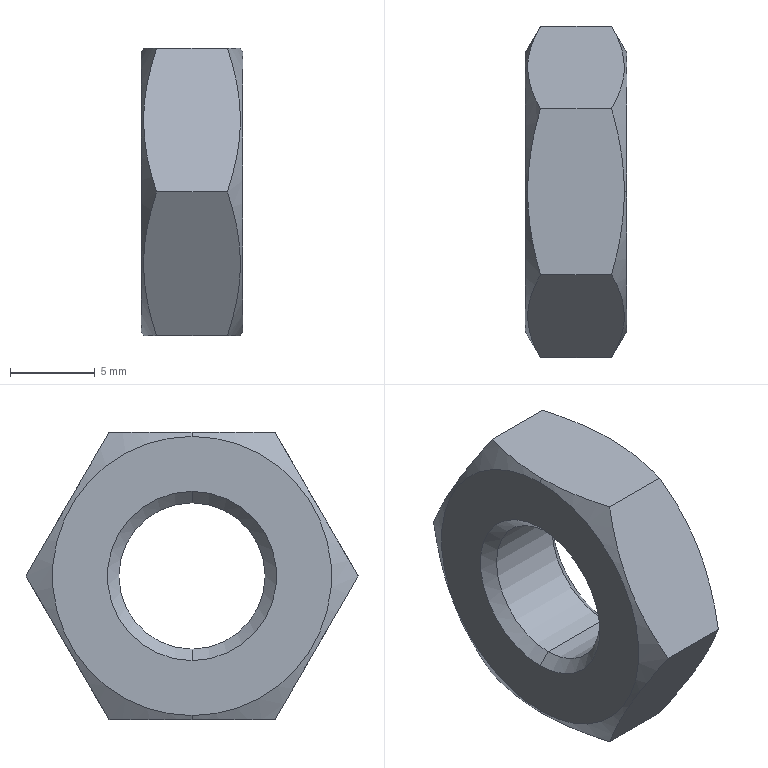Part | SolidWorks | features BaseBody 1 | 1 solid | 18 faces | box 6 x 19.63 x 17 mm | volume 1117 mm3 | cone 8 | plane 8 | cylinder 2 | commonest cylinder face diameters 8.647 x2
STEP:
#1=CARTESIAN_POINT('',(3.,0.,-8.25));
#2=VERTEX_POINT('',#1);
#3=CARTESIAN_POINT('',(3.,0.,8.25));
#4=VERTEX_POINT('',#3);
#5=CARTESIAN_POINT('',(3.,0.,0.));
#6=DIRECTION('',(1.,0.,0.));
#7=DIRECTION('',(0.,0.,1.));
#8=AXIS2_PLACEMENT_3D('',#5,#6,#7);
#9=CIRCLE('',#8,8.25);
#10=EDGE_CURVE('',#2,#4,#9,.T.);
#11=ORIENTED_EDGE('',*,*,#10,.F.);
#12=CARTESIAN_POINT('',(2.856,0.,-8.5));
#13=VERTEX_POINT('',#12);
#14=CARTESIAN_POINT('',(2.091,0.,-9.824));
#15=DIRECTION('',(-0.5,0.,-0.866));
#16=VECTOR('',#15,1000.);
#17=LINE('',#14,#16);
#18=EDGE_CURVE('',#2,#13,#17,.T.);
#19=ORIENTED_EDGE('',*,*,#18,.T.);
#20=CARTESIAN_POINT('',(2.096,4.907,-8.5));
#21=VERTEX_POINT('',#20);
#22=CARTESIAN_POINT('',(2.856,0.,-8.5));
#23=CARTESIAN_POINT('',(2.856,0.4165,-8.5));
#24=CARTESIAN_POINT('',(2.838,0.8348,-8.5));
#25=CARTESIAN_POINT('',(2.768,1.662,-8.5));
#26=CARTESIAN_POINT('',(2.717,2.073,-8.5));
#27=CARTESIAN_POINT('',(2.518,3.299,-8.5));
#28=CARTESIAN_POINT('',(2.328,4.107,-8.5));
#29=CARTESIAN_POINT('',(2.096,4.907,-8.5));
#30=B_SPLINE_CURVE_WITH_KNOTS('',3,(#22,#23,#24,#25,#26,#27,#28,#29),.UNSPECIFIED.,.F.,.F.,(4,2,2,4),(0.004966,0.006202,0.007439,0.009913),.UNSPECIFIED.);
#31=EDGE_CURVE('',#13,#21,#30,.T.);
#32=ORIENTED_EDGE('',*,*,#31,.T.);
#33=CARTESIAN_POINT('',(2.096,9.815,-0.000000029));
#34=VERTEX_POINT('',#33);
#35=CARTESIAN_POINT('',(2.096,4.907,-8.5));
#36=CARTESIAN_POINT('',(2.328,5.308,-7.806));
#37=CARTESIAN_POINT('',(2.518,5.712,-7.107));
#38=CARTESIAN_POINT('',(2.783,6.527,-5.694));
#39=CARTESIAN_POINT('',(2.855,6.939,-4.981));
#40=CARTESIAN_POINT('',(2.856,7.565,-3.897));
#41=CARTESIAN_POINT('',(2.838,7.775,-3.534));
#42=CARTESIAN_POINT('',(2.769,8.189,-2.816));
#43=CARTESIAN_POINT('',(2.718,8.395,-2.459));
#44=CARTESIAN_POINT('',(2.519,9.009,-1.395));
#45=CARTESIAN_POINT('',(2.328,9.414,-0.6948));
#46=CARTESIAN_POINT('',(2.096,9.815,-0.000000029));
#47=B_SPLINE_CURVE_WITH_KNOTS('',3,(#35,#36,#37,#38,#39,#40,#41,#42,#43,#44,#45,#46),.UNSPECIFIED.,.F.,.F.,(4,2,2,2,2,4),(0.,0.002478,0.004956,0.006195,0.007434,0.009913),.UNSPECIFIED.);
#48=EDGE_CURVE('',#21,#34,#47,.T.);
#49=ORIENTED_EDGE('',*,*,#48,.T.);
#50=CARTESIAN_POINT('',(2.096,4.907,8.5));
#51=VERTEX_POINT('',#50);
#52=CARTESIAN_POINT('',(2.096,9.815,-0.000000029));
#53=CARTESIAN_POINT('',(2.328,9.414,0.6939));
#54=CARTESIAN_POINT('',(2.518,9.011,1.393));
#55=CARTESIAN_POINT('',(2.783,8.195,2.806));
#56=CARTESIAN_POINT('',(2.855,7.783,3.519));
#57=CARTESIAN_POINT('',(2.856,7.157,4.603));
#58=CARTESIAN_POINT('',(2.838,6.948,4.966));
#59=CARTESIAN_POINT('',(2.769,6.533,5.684));
#60=CARTESIAN_POINT('',(2.718,6.327,6.041));
#61=CARTESIAN_POINT('',(2.519,5.713,7.105));
#62=CARTESIAN_POINT('',(2.328,5.309,7.805));
#63=CARTESIAN_POINT('',(2.096,4.907,8.5));
#64=B_SPLINE_CURVE_WITH_KNOTS('',3,(#52,#53,#54,#55,#56,#57,#58,#59,#60,#61,#62,#63),.UNSPECIFIED.,.F.,.F.,(4,2,2,2,2,4),(0.,0.002478,0.004956,0.006195,0.007434,0.009913),.UNSPECIFIED.);
#65=EDGE_CURVE('',#34,#51,#64,.T.);
#66=ORIENTED_EDGE('',*,*,#65,.T.);
#67=CARTESIAN_POINT('',(2.856,0.,8.5));
#68=VERTEX_POINT('',#67);
#69=CARTESIAN_POINT('',(2.096,4.907,8.5));
#70=CARTESIAN_POINT('',(2.328,4.105,8.5));
#71=CARTESIAN_POINT('',(2.519,3.296,8.5));
#72=CARTESIAN_POINT('',(2.783,1.662,8.5));
#73=CARTESIAN_POINT('',(2.856,0.8361,8.5));
#74=CARTESIAN_POINT('',(2.856,0.,8.5));
#75=B_SPLINE_CURVE_WITH_KNOTS('',3,(#69,#70,#71,#72,#73,#74),.UNSPECIFIED.,.F.,.F.,(4,2,4),(0.,0.002483,0.004966),.UNSPECIFIED.);
#76=EDGE_CURVE('',#51,#68,#75,.T.);
#77=ORIENTED_EDGE('',*,*,#76,.T.);
#78=CARTESIAN_POINT('',(2.091,0.,9.824));
#79=DIRECTION('',(-0.5,0.,0.866));
#80=VECTOR('',#79,1000.);
#81=LINE('',#78,#80);
#82=EDGE_CURVE('',#4,#68,#81,.T.);
#83=ORIENTED_EDGE('',*,*,#82,.F.);
#84=EDGE_LOOP('',(#11,#19,#32,#49,#66,#77,#83));
#85=FACE_OUTER_BOUND('',#84,.T.);
#86=CARTESIAN_POINT('',(2.091,0.,0.));
#87=DIRECTION('',(-1.,0.,0.));
#88=DIRECTION('',(0.,0.,1.));
#89=AXIS2_PLACEMENT_3D('',#86,#87,#88);
#90=CONICAL_SURFACE('',#89,9.824,1.047);
#91=ADVANCED_FACE('',(#85),#90,.T.);
#92=CARTESIAN_POINT('',(2.323,0.,4.323));
#93=VERTEX_POINT('',#92);
#94=CARTESIAN_POINT('',(2.323,0.,-4.323));
#95=VERTEX_POINT('',#94);
#96=CARTESIAN_POINT('',(2.323,0.,0.));
#97=DIRECTION('',(1.,0.,0.));
#98=DIRECTION('',(0.,0.,-1.));
#99=AXIS2_PLACEMENT_3D('',#96,#97,#98);
#100=CIRCLE('',#99,4.323);
#101=EDGE_CURVE('',#93,#95,#100,.T.);
#102=ORIENTED_EDGE('',*,*,#101,.F.);
#103=CARTESIAN_POINT('',(3.,0.,5.));
#104=VERTEX_POINT('',#103);
#105=CARTESIAN_POINT('',(3.,0.,5.));
#106=DIRECTION('',(0.7071,0.,0.7071));
#107=VECTOR('',#106,1000.);
#108=LINE('',#105,#107);
#109=EDGE_CURVE('',#93,#104,#108,.T.);
#110=ORIENTED_EDGE('',*,*,#109,.T.);
#111=CARTESIAN_POINT('',(3.,0.,-5.));
#112=VERTEX_POINT('',#111);
#113=CARTESIAN_POINT('',(3.,0.,0.));
#114=DIRECTION('',(-1.,0.,0.));
#115=DIRECTION('',(0.,0.,-1.));
#116=AXIS2_PLACEMENT_3D('',#113,#114,#115);
#117=CIRCLE('',#116,5.);
#118=EDGE_CURVE('',#112,#104,#117,.T.);
#119=ORIENTED_EDGE('',*,*,#118,.F.);
#120=CARTESIAN_POINT('',(3.,0.,-5.));
#121=DIRECTION('',(0.7071,0.,-0.7071));
#122=VECTOR('',#121,1000.);
#123=LINE('',#120,#122);
#124=EDGE_CURVE('',#95,#112,#123,.T.);
#125=ORIENTED_EDGE('',*,*,#124,.F.);
#126=EDGE_LOOP('',(#102,#110,#119,#125));
#127=FACE_OUTER_BOUND('',#126,.T.);
#128=CARTESIAN_POINT('',(3.,0.,0.));
#129=DIRECTION('',(1.,0.,0.));
#130=DIRECTION('',(0.,0.,-1.));
#131=AXIS2_PLACEMENT_3D('',#128,#129,#130);
#132=CONICAL_SURFACE('',#131,5.,0.7854);
#133=ADVANCED_FACE('',(#127),#132,.F.);
#134=CARTESIAN_POINT('',(-2.324,0.,4.324));
#135=VERTEX_POINT('',#134);
#136=CARTESIAN_POINT('',(-2.324,0.,-4.324));
#137=VERTEX_POINT('',#136);
#138=CARTESIAN_POINT('',(-2.324,0.,0.));
#139=DIRECTION('',(1.,0.,0.));
#140=DIRECTION('',(0.,0.,-1.));
#141=AXIS2_PLACEMENT_3D('',#138,#139,#140);
#142=CIRCLE('',#141,4.324);
#143=EDGE_CURVE('',#135,#137,#142,.T.);
#144=ORIENTED_EDGE('',*,*,#143,.F.);
#145=CARTESIAN_POINT('',(3.,0.,4.324));
#146=DIRECTION('',(1.,0.,0.));
#147=VECTOR('',#146,1000.);
#148=LINE('',#145,#147);
#149=EDGE_CURVE('',#135,#93,#148,.T.);
#150=ORIENTED_EDGE('',*,*,#149,.T.);
#151=ORIENTED_EDGE('',*,*,#101,.T.);
#152=CARTESIAN_POINT('',(3.,0.,-4.324));
#153=DIRECTION('',(1.,0.,0.));
#154=VECTOR('',#153,1000.);
#155=LINE('',#152,#154);
#156=EDGE_CURVE('',#137,#95,#155,.T.);
#157=ORIENTED_EDGE('',*,*,#156,.F.);
#158=EDGE_LOOP('',(#144,#150,#151,#157));
#159=FACE_OUTER_BOUND('',#158,.T.);
#160=CARTESIAN_POINT('',(3.,0.,0.));
#161=DIRECTION('',(1.,0.,0.));
#162=DIRECTION('',(0.,0.,-1.));
#163=AXIS2_PLACEMENT_3D('',#160,#161,#162);
#164=CYLINDRICAL_SURFACE('',#163,4.324);
#165=ADVANCED_FACE('',(#159),#164,.F.);
#166=CARTESIAN_POINT('',(-3.,0.,-8.25));
#167=VERTEX_POINT('',#166);
#168=CARTESIAN_POINT('',(-3.,0.,8.25));
#169=VERTEX_POINT('',#168);
#170=CARTESIAN_POINT('',(-3.,0.,0.));
#171=DIRECTION('',(1.,0.,0.));
#172=DIRECTION('',(0.,0.,-1.));
#173=AXIS2_PLACEMENT_3D('',#170,#171,#172);
#174=CIRCLE('',#173,8.25);
#175=EDGE_CURVE('',#167,#169,#174,.T.);
#176=ORIENTED_EDGE('',*,*,#175,.T.);
#177=CARTESIAN_POINT('',(-2.856,0.,8.5));
#178=VERTEX_POINT('',#177);
#179=CARTESIAN_POINT('',(-2.091,0.,9.824));
#180=DIRECTION('',(0.5,0.,0.866));
#181=VECTOR('',#180,1000.);
#182=LINE('',#179,#181);
#183=EDGE_CURVE('',#169,#178,#182,.T.);
#184=ORIENTED_EDGE('',*,*,#183,.T.);
#185=CARTESIAN_POINT('',(-2.096,4.907,8.5));
#186=VERTEX_POINT('',#185);
#187=CARTESIAN_POINT('',(-2.856,0.,8.5));
#188=CARTESIAN_POINT('',(-2.856,0.4165,8.5));
#189=CARTESIAN_POINT('',(-2.838,0.8348,8.5));
#190=CARTESIAN_POINT('',(-2.768,1.662,8.5));
#191=CARTESIAN_POINT('',(-2.717,2.073,8.5));
#192=CARTESIAN_POINT('',(-2.518,3.299,8.5));
#193=CARTESIAN_POINT('',(-2.328,4.107,8.5));
#194=CARTESIAN_POINT('',(-2.096,4.907,8.5));
#195=B_SPLINE_CURVE_WITH_KNOTS('',3,(#187,#188,#189,#190,#191,#192,#193,#194),.UNSPECIFIED.,.F.,.F.,(4,2,2,4),(0.004966,0.006202,0.007439,0.009913),.UNSPECIFIED.);
#196=EDGE_CURVE('',#178,#186,#195,.T.);
#197=ORIENTED_EDGE('',*,*,#196,.T.);
#198=CARTESIAN_POINT('',(-2.096,9.815,0.));
#199=VERTEX_POINT('',#198);
#200=CARTESIAN_POINT('',(-2.096,4.907,8.5));
#201=CARTESIAN_POINT('',(-2.328,5.308,7.806));
#202=CARTESIAN_POINT('',(-2.518,5.712,7.107));
#203=CARTESIAN_POINT('',(-2.783,6.527,5.694));
#204=CARTESIAN_POINT('',(-2.855,6.939,4.981));
#205=CARTESIAN_POINT('',(-2.856,7.565,3.897));
#206=CARTESIAN_POINT('',(-2.838,7.775,3.534));
#207=CARTESIAN_POINT('',(-2.769,8.189,2.816));
#208=CARTESIAN_POINT('',(-2.718,8.395,2.459));
#209=CARTESIAN_POINT('',(-2.519,9.009,1.395));
#210=CARTESIAN_POINT('',(-2.328,9.414,0.6948));
#211=CARTESIAN_POINT('',(-2.096,9.815,0.));
#212=B_SPLINE_CURVE_WITH_KNOTS('',3,(#200,#201,#202,#203,#204,#205,#206,#207,#208,#209,#210,#211),.UNSPECIFIED.,.F.,.F.,(4,2,2,2,2,4),(0.,0.002478,0.004956,0.006195,0.007434,0.009913),.UNSPECIFIED.);
#213=EDGE_CURVE('',#186,#199,#212,.T.);
#214=ORIENTED_EDGE('',*,*,#213,.T.);
#215=CARTESIAN_POINT('',(-2.096,4.907,-8.5));
#216=VERTEX_POINT('',#215);
#217=CARTESIAN_POINT('',(-2.096,9.815,0.));
#218=CARTESIAN_POINT('',(-2.328,9.414,-0.6939));
#219=CARTESIAN_POINT('',(-2.518,9.011,-1.393));
#220=CARTESIAN_POINT('',(-2.783,8.195,-2.806));
#221=CARTESIAN_POINT('',(-2.855,7.783,-3.519));
#222=CARTESIAN_POINT('',(-2.856,7.157,-4.603));
#223=CARTESIAN_POINT('',(-2.838,6.948,-4.966));
#224=CARTESIAN_POINT('',(-2.769,6.533,-5.684));
#225=CARTESIAN_POINT('',(-2.718,6.327,-6.041));
#226=CARTESIAN_POINT('',(-2.519,5.713,-7.105));
#227=CARTESIAN_POINT('',(-2.328,5.309,-7.805));
#228=CARTESIAN_POINT('',(-2.096,4.907,-8.5));
#229=B_SPLINE_CURVE_WITH_KNOTS('',3,(#217,#218,#219,#220,#221,#222,#223,#224,#225,#226,#227,#228),.UNSPECIFIED.,.F.,.F.,(4,2,2,2,2,4),(0.,0.002478,0.004956,0.006195,0.007434,0.009913),.UNSPECIFIED.);
#230=EDGE_CURVE('',#199,#216,#229,.T.);
#231=ORIENTED_EDGE('',*,*,#230,.T.);
#232=CARTESIAN_POINT('',(-2.856,0.,-8.5));
#233=VERTEX_POINT('',#232);
#234=CARTESIAN_POINT('',(-2.096,4.907,-8.5));
#235=CARTESIAN_POINT('',(-2.328,4.105,-8.5));
#236=CARTESIAN_POINT('',(-2.519,3.296,-8.5));
#237=CARTESIAN_POINT('',(-2.783,1.662,-8.5));
#238=CARTESIAN_POINT('',(-2.856,0.8361,-8.5));
#239=CARTESIAN_POINT('',(-2.856,0.,-8.5));
#240=B_SPLINE_CURVE_WITH_KNOTS('',3,(#234,#235,#236,#237,#238,#239),.UNSPECIFIED.,.F.,.F.,(4,2,4),(0.,0.002483,0.004966),.UNSPECIFIED.);
#241=EDGE_CURVE('',#216,#233,#240,.T.);
#242=ORIENTED_EDGE('',*,*,#241,.T.);
#243=CARTESIAN_POINT('',(-2.091,0.,-9.824));
#244=DIRECTION('',(0.5,0.,-0.866));
#245=VECTOR('',#244,1000.);
#246=LINE('',#243,#245);
#247=EDGE_CURVE('',#167,#233,#246,.T.);
#248=ORIENTED_EDGE('',*,*,#247,.F.);
#249=EDGE_LOOP('',(#176,#184,#197,#214,#231,#242,#248));
#250=FACE_OUTER_BOUND('',#249,.T.);
#251=CARTESIAN_POINT('',(-2.091,0.,0.));
#252=DIRECTION('',(1.,0.,0.));
#253=DIRECTION('',(0.,0.,-1.));
#254=AXIS2_PLACEMENT_3D('',#251,#252,#253);
#255=CONICAL_SURFACE('',#254,9.824,1.047);
#256=ADVANCED_FACE('',(#250),#255,.T.);
#257=ORIENTED_EDGE('',*,*,#143,.T.);
#258=CARTESIAN_POINT('',(-3.,0.,-5.));
#259=VERTEX_POINT('',#258);
#260=CARTESIAN_POINT('',(-3.,0.,-5.));
#261=DIRECTION('',(-0.7071,0.,-0.7071));
#262=VECTOR('',#261,1000.);
#263=LINE('',#260,#262);
#264=EDGE_CURVE('',#137,#259,#263,.T.);
#265=ORIENTED_EDGE('',*,*,#264,.T.);
#266=CARTESIAN_POINT('',(-3.,0.,5.));
#267=VERTEX_POINT('',#266);
#268=CARTESIAN_POINT('',(-3.,0.,0.));
#269=DIRECTION('',(1.,0.,0.));
#270=DIRECTION('',(0.,0.,1.));
#271=AXIS2_PLACEMENT_3D('',#268,#269,#270);
#272=CIRCLE('',#271,5.);
#273=EDGE_CURVE('',#267,#259,#272,.T.);
#274=ORIENTED_EDGE('',*,*,#273,.F.);
#275=CARTESIAN_POINT('',(-3.,0.,5.));
#276=DIRECTION('',(-0.7071,0.,0.7071));
#277=VECTOR('',#276,1000.);
#278=LINE('',#275,#277);
#279=EDGE_CURVE('',#135,#267,#278,.T.);
#280=ORIENTED_EDGE('',*,*,#279,.F.);
#281=EDGE_LOOP('',(#257,#265,#274,#280));
#282=FACE_OUTER_BOUND('',#281,.T.);
#283=CARTESIAN_POINT('',(-3.,0.,0.));
#284=DIRECTION('',(-1.,0.,0.));
#285=DIRECTION('',(0.,0.,1.));
#286=AXIS2_PLACEMENT_3D('',#283,#284,#285);
#287=CONICAL_SURFACE('',#286,5.,0.7854);
#288=ADVANCED_FACE('',(#282),#287,.F.);
#289=CARTESIAN_POINT('',(3.,0.,0.));
#290=DIRECTION('',(1.,0.,0.));
#291=DIRECTION('',(0.,0.,1.));
#292=AXIS2_PLACEMENT_3D('',#289,#290,#291);
#293=CIRCLE('',#292,8.25);
#294=EDGE_CURVE('',#4,#2,#293,.T.);
#295=ORIENTED_EDGE('',*,*,#294,.T.);
#296=ORIENTED_EDGE('',*,*,#10,.T.);
#297=EDGE_LOOP('',(#295,#296));
#298=FACE_OUTER_BOUND('',#297,.T.);
#299=ORIENTED_EDGE('',*,*,#118,.T.);
#300=CARTESIAN_POINT('',(3.,0.,0.));
#301=DIRECTION('',(-1.,0.,0.));
#302=DIRECTION('',(0.,0.,-1.));
#303=AXIS2_PLACEMENT_3D('',#300,#301,#302);
#304=CIRCLE('',#303,5.);
#305=EDGE_CURVE('',#104,#112,#304,.T.);
#306=ORIENTED_EDGE('',*,*,#305,.T.);
#307=EDGE_LOOP('',(#299,#306));
#308=FACE_BOUND('',#307,.T.);
#309=CARTESIAN_POINT('',(3.,0.,0.));
#310=DIRECTION('',(1.,0.,0.));
#311=DIRECTION('',(0.,0.,-1.));
#312=AXIS2_PLACEMENT_3D('',#309,#310,#311);
#313=PLANE('',#312);
#314=ADVANCED_FACE('',(#298,#308),#313,.T.);
#315=ORIENTED_EDGE('',*,*,#18,.F.);
#316=ORIENTED_EDGE('',*,*,#294,.F.);
#317=ORIENTED_EDGE('',*,*,#82,.T.);
#318=CARTESIAN_POINT('',(2.096,-4.907,8.5));
#319=VERTEX_POINT('',#318);
#320=CARTESIAN_POINT('',(2.856,0.,8.5));
#321=CARTESIAN_POINT('',(2.856,-0.4165,8.5));
#322=CARTESIAN_POINT('',(2.838,-0.8348,8.5));
#323=CARTESIAN_POINT('',(2.768,-1.662,8.5));
#324=CARTESIAN_POINT('',(2.717,-2.073,8.5));
#325=CARTESIAN_POINT('',(2.518,-3.299,8.5));
#326=CARTESIAN_POINT('',(2.328,-4.107,8.5));
#327=CARTESIAN_POINT('',(2.096,-4.907,8.5));
#328=B_SPLINE_CURVE_WITH_KNOTS('',3,(#320,#321,#322,#323,#324,#325,#326,#327),.UNSPECIFIED.,.F.,.F.,(4,2,2,4),(0.004966,0.006202,0.007439,0.009913),.UNSPECIFIED.);
#329=EDGE_CURVE('',#68,#319,#328,.T.);
#330=ORIENTED_EDGE('',*,*,#329,.T.);
#331=CARTESIAN_POINT('',(2.096,-9.815,0.000000029));
#332=VERTEX_POINT('',#331);
#333=CARTESIAN_POINT('',(2.096,-4.907,8.5));
#334=CARTESIAN_POINT('',(2.328,-5.308,7.806));
#335=CARTESIAN_POINT('',(2.518,-5.712,7.107));
#336=CARTESIAN_POINT('',(2.783,-6.527,5.694));
#337=CARTESIAN_POINT('',(2.855,-6.939,4.981));
#338=CARTESIAN_POINT('',(2.856,-7.565,3.897));
#339=CARTESIAN_POINT('',(2.838,-7.775,3.534));
#340=CARTESIAN_POINT('',(2.769,-8.189,2.816));
#341=CARTESIAN_POINT('',(2.718,-8.395,2.459));
#342=CARTESIAN_POINT('',(2.519,-9.009,1.395));
#343=CARTESIAN_POINT('',(2.328,-9.414,0.6948));
#344=CARTESIAN_POINT('',(2.096,-9.815,0.000000029));
#345=B_SPLINE_CURVE_WITH_KNOTS('',3,(#333,#334,#335,#336,#337,#338,#339,#340,#341,#342,#343,#344),.UNSPECIFIED.,.F.,.F.,(4,2,2,2,2,4),(0.,0.002478,0.004956,0.006195,0.007434,0.009913),.UNSPECIFIED.);
#346=EDGE_CURVE('',#319,#332,#345,.T.);
#347=ORIENTED_EDGE('',*,*,#346,.T.);
#348=CARTESIAN_POINT('',(2.096,-4.907,-8.5));
#349=VERTEX_POINT('',#348);
#350=CARTESIAN_POINT('',(2.096,-9.815,0.000000029));
#351=CARTESIAN_POINT('',(2.328,-9.414,-0.6939));
#352=CARTESIAN_POINT('',(2.518,-9.011,-1.393));
#353=CARTESIAN_POINT('',(2.783,-8.195,-2.806));
#354=CARTESIAN_POINT('',(2.855,-7.783,-3.519));
#355=CARTESIAN_POINT('',(2.856,-7.157,-4.603));
#356=CARTESIAN_POINT('',(2.838,-6.948,-4.966));
#357=CARTESIAN_POINT('',(2.769,-6.533,-5.684));
#358=CARTESIAN_POINT('',(2.718,-6.327,-6.041));
#359=CARTESIAN_POINT('',(2.519,-5.713,-7.105));
#360=CARTESIAN_POINT('',(2.328,-5.309,-7.805));
#361=CARTESIAN_POINT('',(2.096,-4.907,-8.5));
#362=B_SPLINE_CURVE_WITH_KNOTS('',3,(#350,#351,#352,#353,#354,#355,#356,#357,#358,#359,#360,#361),.UNSPECIFIED.,.F.,.F.,(4,2,2,2,2,4),(0.,0.002478,0.004956,0.006195,0.007434,0.009913),.UNSPECIFIED.);
#363=EDGE_CURVE('',#332,#349,#362,.T.);
#364=ORIENTED_EDGE('',*,*,#363,.T.);
#365=CARTESIAN_POINT('',(2.096,-4.907,-8.5));
#366=CARTESIAN_POINT('',(2.328,-4.105,-8.5));
#367=CARTESIAN_POINT('',(2.519,-3.296,-8.5));
#368=CARTESIAN_POINT('',(2.783,-1.662,-8.5));
#369=CARTESIAN_POINT('',(2.856,-0.8361,-8.5));
#370=CARTESIAN_POINT('',(2.856,0.,-8.5));
#371=B_SPLINE_CURVE_WITH_KNOTS('',3,(#365,#366,#367,#368,#369,#370),.UNSPECIFIED.,.F.,.F.,(4,2,4),(0.,0.002483,0.004966),.UNSPECIFIED.);
#372=EDGE_CURVE('',#349,#13,#371,.T.);
#373=ORIENTED_EDGE('',*,*,#372,.T.);
#374=EDGE_LOOP('',(#315,#316,#317,#330,#347,#364,#373));
#375=FACE_OUTER_BOUND('',#374,.T.);
#376=CARTESIAN_POINT('',(2.091,0.,0.));
#377=DIRECTION('',(-1.,0.,0.));
#378=DIRECTION('',(0.,0.,1.));
#379=AXIS2_PLACEMENT_3D('',#376,#377,#378);
#380=CONICAL_SURFACE('',#379,9.824,1.047);
#381=ADVANCED_FACE('',(#375),#380,.T.);
#382=ORIENTED_EDGE('',*,*,#109,.F.);
#383=CARTESIAN_POINT('',(2.323,0.,0.));
#384=DIRECTION('',(1.,0.,0.));
#385=DIRECTION('',(0.,0.,-1.));
#386=AXIS2_PLACEMENT_3D('',#383,#384,#385);
#387=CIRCLE('',#386,4.323);
#388=EDGE_CURVE('',#95,#93,#387,.T.);
#389=ORIENTED_EDGE('',*,*,#388,.F.);
#390=ORIENTED_EDGE('',*,*,#124,.T.);
#391=ORIENTED_EDGE('',*,*,#305,.F.);
#392=EDGE_LOOP('',(#382,#389,#390,#391));
#393=FACE_OUTER_BOUND('',#392,.T.);
#394=CARTESIAN_POINT('',(3.,0.,0.));
#395=DIRECTION('',(1.,0.,0.));
#396=DIRECTION('',(0.,0.,-1.));
#397=AXIS2_PLACEMENT_3D('',#394,#395,#396);
#398=CONICAL_SURFACE('',#397,5.,0.7854);
#399=ADVANCED_FACE('',(#393),#398,.F.);
#400=CARTESIAN_POINT('',(-2.096,-4.907,8.5));
#401=VERTEX_POINT('',#400);
#402=CARTESIAN_POINT('',(-2.096,-4.907,8.5));
#403=CARTESIAN_POINT('',(-2.328,-4.105,8.5));
#404=CARTESIAN_POINT('',(-2.519,-3.296,8.5));
#405=CARTESIAN_POINT('',(-2.783,-1.662,8.5));
#406=CARTESIAN_POINT('',(-2.856,-0.8361,8.5));
#407=CARTESIAN_POINT('',(-2.856,0.,8.5));
#408=B_SPLINE_CURVE_WITH_KNOTS('',3,(#402,#403,#404,#405,#406,#407),.UNSPECIFIED.,.F.,.F.,(4,2,4),(0.,0.002483,0.004966),.UNSPECIFIED.);
#409=EDGE_CURVE('',#401,#178,#408,.T.);
#410=ORIENTED_EDGE('',*,*,#409,.F.);
#411=CARTESIAN_POINT('',(3.,-4.907,8.5));
#412=DIRECTION('',(-1.,0.,0.));
#413=VECTOR('',#412,1000.);
#414=LINE('',#411,#413);
#415=EDGE_CURVE('',#319,#401,#414,.T.);
#416=ORIENTED_EDGE('',*,*,#415,.F.);
#417=ORIENTED_EDGE('',*,*,#329,.F.);
#418=ORIENTED_EDGE('',*,*,#76,.F.);
#419=CARTESIAN_POINT('',(3.,4.907,8.5));
#420=DIRECTION('',(1.,0.,0.));
#421=VECTOR('',#420,1000.);
#422=LINE('',#419,#421);
#423=EDGE_CURVE('',#186,#51,#422,.T.);
#424=ORIENTED_EDGE('',*,*,#423,.F.);
#425=ORIENTED_EDGE('',*,*,#196,.F.);
#426=EDGE_LOOP('',(#410,#416,#417,#418,#424,#425));
#427=FACE_OUTER_BOUND('',#426,.T.);
#428=CARTESIAN_POINT('',(3.,4.907,8.5));
#429=DIRECTION('',(0.,0.,-1.));
#430=DIRECTION('',(-1.,0.,0.));
#431=AXIS2_PLACEMENT_3D('',#428,#429,#430);
#432=PLANE('',#431);
#433=ADVANCED_FACE('',(#427),#432,.F.);
#434=ORIENTED_EDGE('',*,*,#213,.F.);
#435=ORIENTED_EDGE('',*,*,#423,.T.);
#436=ORIENTED_EDGE('',*,*,#65,.F.);
#437=CARTESIAN_POINT('',(3.,9.815,0.));
#438=DIRECTION('',(1.,0.,0.));
#439=VECTOR('',#438,1000.);
#440=LINE('',#437,#439);
#441=EDGE_CURVE('',#199,#34,#440,.T.);
#442=ORIENTED_EDGE('',*,*,#441,.F.);
#443=EDGE_LOOP('',(#434,#435,#436,#442));
#444=FACE_OUTER_BOUND('',#443,.T.);
#445=CARTESIAN_POINT('',(3.,9.815,0.));
#446=DIRECTION('',(0.,-0.866,-0.5));
#447=DIRECTION('',(0.,0.5,-0.866));
#448=AXIS2_PLACEMENT_3D('',#445,#446,#447);
#449=PLANE('',#448);
#450=ADVANCED_FACE('',(#444),#449,.F.);
#451=ORIENTED_EDGE('',*,*,#230,.F.);
#452=ORIENTED_EDGE('',*,*,#441,.T.);
#453=ORIENTED_EDGE('',*,*,#48,.F.);
#454=CARTESIAN_POINT('',(3.,4.907,-8.5));
#455=DIRECTION('',(1.,0.,0.));
#456=VECTOR('',#455,1000.);
#457=LINE('',#454,#456);
#458=EDGE_CURVE('',#216,#21,#457,.T.);
#459=ORIENTED_EDGE('',*,*,#458,.F.);
#460=EDGE_LOOP('',(#451,#452,#453,#459));
#461=FACE_OUTER_BOUND('',#460,.T.);
#462=CARTESIAN_POINT('',(3.,4.907,-8.5));
#463=DIRECTION('',(0.,-0.866,0.5));
#464=DIRECTION('',(0.,-0.5,-0.866));
#465=AXIS2_PLACEMENT_3D('',#462,#463,#464);
#466=PLANE('',#465);
#467=ADVANCED_FACE('',(#461),#466,.F.);
#468=ORIENTED_EDGE('',*,*,#241,.F.);
#469=ORIENTED_EDGE('',*,*,#458,.T.);
#470=ORIENTED_EDGE('',*,*,#31,.F.);
#471=ORIENTED_EDGE('',*,*,#372,.F.);
#472=CARTESIAN_POINT('',(-2.096,-4.907,-8.5));
#473=VERTEX_POINT('',#472);
#474=CARTESIAN_POINT('',(3.,-4.907,-8.5));
#475=DIRECTION('',(1.,0.,0.));
#476=VECTOR('',#475,1000.);
#477=LINE('',#474,#476);
#478=EDGE_CURVE('',#473,#349,#477,.T.);
#479=ORIENTED_EDGE('',*,*,#478,.F.);
#480=CARTESIAN_POINT('',(-2.856,0.,-8.5));
#481=CARTESIAN_POINT('',(-2.856,-0.4165,-8.5));
#482=CARTESIAN_POINT('',(-2.838,-0.8348,-8.5));
#483=CARTESIAN_POINT('',(-2.768,-1.662,-8.5));
#484=CARTESIAN_POINT('',(-2.717,-2.073,-8.5));
#485=CARTESIAN_POINT('',(-2.518,-3.299,-8.5));
#486=CARTESIAN_POINT('',(-2.328,-4.107,-8.5));
#487=CARTESIAN_POINT('',(-2.096,-4.907,-8.5));
#488=B_SPLINE_CURVE_WITH_KNOTS('',3,(#480,#481,#482,#483,#484,#485,#486,#487),.UNSPECIFIED.,.F.,.F.,(4,2,2,4),(0.004966,0.006202,0.007439,0.009913),.UNSPECIFIED.);
#489=EDGE_CURVE('',#233,#473,#488,.T.);
#490=ORIENTED_EDGE('',*,*,#489,.F.);
#491=EDGE_LOOP('',(#468,#469,#470,#471,#479,#490));
#492=FACE_OUTER_BOUND('',#491,.T.);
#493=CARTESIAN_POINT('',(3.,-4.907,-8.5));
#494=DIRECTION('',(0.,0.,1.));
#495=DIRECTION('',(1.,0.,0.));
#496=AXIS2_PLACEMENT_3D('',#493,#494,#495);
#497=PLANE('',#496);
#498=ADVANCED_FACE('',(#492),#497,.F.);
#499=CARTESIAN_POINT('',(-2.096,-9.815,0.));
#500=VERTEX_POINT('',#499);
#501=CARTESIAN_POINT('',(-2.096,-4.907,-8.5));
#502=CARTESIAN_POINT('',(-2.328,-5.308,-7.806));
#503=CARTESIAN_POINT('',(-2.518,-5.712,-7.107));
#504=CARTESIAN_POINT('',(-2.783,-6.527,-5.694));
#505=CARTESIAN_POINT('',(-2.855,-6.939,-4.981));
#506=CARTESIAN_POINT('',(-2.856,-7.565,-3.897));
#507=CARTESIAN_POINT('',(-2.838,-7.775,-3.534));
#508=CARTESIAN_POINT('',(-2.769,-8.189,-2.816));
#509=CARTESIAN_POINT('',(-2.718,-8.395,-2.459));
#510=CARTESIAN_POINT('',(-2.519,-9.009,-1.395));
#511=CARTESIAN_POINT('',(-2.328,-9.414,-0.6948));
#512=CARTESIAN_POINT('',(-2.096,-9.815,0.));
#513=B_SPLINE_CURVE_WITH_KNOTS('',3,(#501,#502,#503,#504,#505,#506,#507,#508,#509,#510,#511,#512),.UNSPECIFIED.,.F.,.F.,(4,2,2,2,2,4),(0.,0.002478,0.004956,0.006195,0.007434,0.009913),.UNSPECIFIED.);
#514=EDGE_CURVE('',#473,#500,#513,.T.);
#515=ORIENTED_EDGE('',*,*,#514,.F.);
#516=ORIENTED_EDGE('',*,*,#478,.T.);
#517=ORIENTED_EDGE('',*,*,#363,.F.);
#518=CARTESIAN_POINT('',(3.,-9.815,0.));
#519=DIRECTION('',(1.,0.,0.));
#520=VECTOR('',#519,1000.);
#521=LINE('',#518,#520);
#522=EDGE_CURVE('',#500,#332,#521,.T.);
#523=ORIENTED_EDGE('',*,*,#522,.F.);
#524=EDGE_LOOP('',(#515,#516,#517,#523));
#525=FACE_OUTER_BOUND('',#524,.T.);
#526=CARTESIAN_POINT('',(3.,-9.815,0.));
#527=DIRECTION('',(0.,0.866,0.5));
#528=DIRECTION('',(0.,-0.5,0.866));
#529=AXIS2_PLACEMENT_3D('',#526,#527,#528);
#530=PLANE('',#529);
#531=ADVANCED_FACE('',(#525),#530,.F.);
#532=CARTESIAN_POINT('',(-2.096,-9.815,0.));
#533=CARTESIAN_POINT('',(-2.328,-9.414,0.6939));
#534=CARTESIAN_POINT('',(-2.518,-9.011,1.393));
#535=CARTESIAN_POINT('',(-2.783,-8.195,2.806));
#536=CARTESIAN_POINT('',(-2.855,-7.783,3.519));
#537=CARTESIAN_POINT('',(-2.856,-7.157,4.603));
#538=CARTESIAN_POINT('',(-2.838,-6.948,4.966));
#539=CARTESIAN_POINT('',(-2.769,-6.533,5.684));
#540=CARTESIAN_POINT('',(-2.718,-6.327,6.041));
#541=CARTESIAN_POINT('',(-2.519,-5.713,7.105));
#542=CARTESIAN_POINT('',(-2.328,-5.309,7.805));
#543=CARTESIAN_POINT('',(-2.096,-4.907,8.5));
#544=B_SPLINE_CURVE_WITH_KNOTS('',3,(#532,#533,#534,#535,#536,#537,#538,#539,#540,#541,#542,#543),.UNSPECIFIED.,.F.,.F.,(4,2,2,2,2,4),(0.,0.002478,0.004956,0.006195,0.007434,0.009913),.UNSPECIFIED.);
#545=EDGE_CURVE('',#500,#401,#544,.T.);
#546=ORIENTED_EDGE('',*,*,#545,.F.);
#547=ORIENTED_EDGE('',*,*,#522,.T.);
#548=ORIENTED_EDGE('',*,*,#346,.F.);
#549=ORIENTED_EDGE('',*,*,#415,.T.);
#550=EDGE_LOOP('',(#546,#547,#548,#549));
#551=FACE_OUTER_BOUND('',#550,.T.);
#552=CARTESIAN_POINT('',(3.,-4.907,8.5));
#553=DIRECTION('',(0.,0.866,-0.5));
#554=DIRECTION('',(0.,0.5,0.866));
#555=AXIS2_PLACEMENT_3D('',#552,#553,#554);
#556=PLANE('',#555);
#557=ADVANCED_FACE('',(#551),#556,.F.);
#558=ORIENTED_EDGE('',*,*,#149,.F.);
#559=CARTESIAN_POINT('',(-2.324,0.,0.));
#560=DIRECTION('',(1.,0.,0.));
#561=DIRECTION('',(0.,0.,-1.));
#562=AXIS2_PLACEMENT_3D('',#559,#560,#561);
#563=CIRCLE('',#562,4.324);
#564=EDGE_CURVE('',#137,#135,#563,.T.);
#565=ORIENTED_EDGE('',*,*,#564,.F.);
#566=ORIENTED_EDGE('',*,*,#156,.T.);
#567=ORIENTED_EDGE('',*,*,#388,.T.);
#568=EDGE_LOOP('',(#558,#565,#566,#567));
#569=FACE_OUTER_BOUND('',#568,.T.);
#570=CARTESIAN_POINT('',(3.,0.,0.));
#571=DIRECTION('',(1.,0.,0.));
#572=DIRECTION('',(0.,0.,-1.));
#573=AXIS2_PLACEMENT_3D('',#570,#571,#572);
#574=CYLINDRICAL_SURFACE('',#573,4.324);
#575=ADVANCED_FACE('',(#569),#574,.F.);
#576=ORIENTED_EDGE('',*,*,#183,.F.);
#577=CARTESIAN_POINT('',(-3.,0.,0.));
#578=DIRECTION('',(1.,0.,0.));
#579=DIRECTION('',(0.,0.,-1.));
#580=AXIS2_PLACEMENT_3D('',#577,#578,#579);
#581=CIRCLE('',#580,8.25);
#582=EDGE_CURVE('',#169,#167,#581,.T.);
#583=ORIENTED_EDGE('',*,*,#582,.T.);
#584=ORIENTED_EDGE('',*,*,#247,.T.);
#585=ORIENTED_EDGE('',*,*,#489,.T.);
#586=ORIENTED_EDGE('',*,*,#514,.T.);
#587=ORIENTED_EDGE('',*,*,#545,.T.);
#588=ORIENTED_EDGE('',*,*,#409,.T.);
#589=EDGE_LOOP('',(#576,#583,#584,#585,#586,#587,#588));
#590=FACE_OUTER_BOUND('',#589,.T.);
#591=CARTESIAN_POINT('',(-2.091,0.,0.));
#592=DIRECTION('',(1.,0.,0.));
#593=DIRECTION('',(0.,0.,-1.));
#594=AXIS2_PLACEMENT_3D('',#591,#592,#593);
#595=CONICAL_SURFACE('',#594,9.824,1.047);
#596=ADVANCED_FACE('',(#590),#595,.T.);
#597=ORIENTED_EDGE('',*,*,#264,.F.);
#598=ORIENTED_EDGE('',*,*,#564,.T.);
#599=ORIENTED_EDGE('',*,*,#279,.T.);
#600=CARTESIAN_POINT('',(-3.,0.,0.));
#601=DIRECTION('',(1.,0.,0.));
#602=DIRECTION('',(0.,0.,1.));
#603=AXIS2_PLACEMENT_3D('',#600,#601,#602);
#604=CIRCLE('',#603,5.);
#605=EDGE_CURVE('',#259,#267,#604,.T.);
#606=ORIENTED_EDGE('',*,*,#605,.F.);
#607=EDGE_LOOP('',(#597,#598,#599,#606));
#608=FACE_OUTER_BOUND('',#607,.T.);
#609=CARTESIAN_POINT('',(-3.,0.,0.));
#610=DIRECTION('',(-1.,0.,0.));
#611=DIRECTION('',(0.,0.,1.));
#612=AXIS2_PLACEMENT_3D('',#609,#610,#611);
#613=CONICAL_SURFACE('',#612,5.,0.7854);
#614=ADVANCED_FACE('',(#608),#613,.F.);
#615=ORIENTED_EDGE('',*,*,#175,.F.);
#616=ORIENTED_EDGE('',*,*,#582,.F.);
#617=EDGE_LOOP('',(#615,#616));
#618=FACE_OUTER_BOUND('',#617,.T.);
#619=ORIENTED_EDGE('',*,*,#273,.T.);
#620=ORIENTED_EDGE('',*,*,#605,.T.);
#621=EDGE_LOOP('',(#619,#620));
#622=FACE_BOUND('',#621,.T.);
#623=CARTESIAN_POINT('',(-3.,0.,0.));
#624=DIRECTION('',(1.,0.,0.));
#625=DIRECTION('',(0.,0.,-1.));
#626=AXIS2_PLACEMENT_3D('',#623,#624,#625);
#627=PLANE('',#626);
#628=ADVANCED_FACE('',(#618,#622),#627,.F.);
#629=CLOSED_SHELL('',(#91,#133,#165,#256,#288,#314,#381,#399,#433,#450,#467,#498,#531,#557,#575,#596,#614,#628));
#630=MANIFOLD_SOLID_BREP('',#629);
#631=CARTESIAN_POINT('',(0.,0.,0.));
#632=DIRECTION('',(0.,0.,1.));
#633=DIRECTION('',(1.,0.,0.));
#634=AXIS2_PLACEMENT_3D('',#631,#632,#633);
#635=(LENGTH_UNIT()NAMED_UNIT(*)SI_UNIT(.MILLI.,.METRE.));
#636=UNCERTAINTY_MEASURE_WITH_UNIT(LENGTH_MEASURE(0.00001),#635,'','');
#637=(NAMED_UNIT(*)PLANE_ANGLE_UNIT()SI_UNIT($,.RADIAN.));
#638=(NAMED_UNIT(*)SI_UNIT($,.STERADIAN.)SOLID_ANGLE_UNIT());
#639=(GEOMETRIC_REPRESENTATION_CONTEXT(3)GLOBAL_UNCERTAINTY_ASSIGNED_CONTEXT((#636))GLOBAL_UNIT_ASSIGNED_CONTEXT((#635,#637,#638))REPRESENTATION_CONTEXT('',''));
#640=ADVANCED_BREP_SHAPE_REPRESENTATION('',(#630,#634),#639);